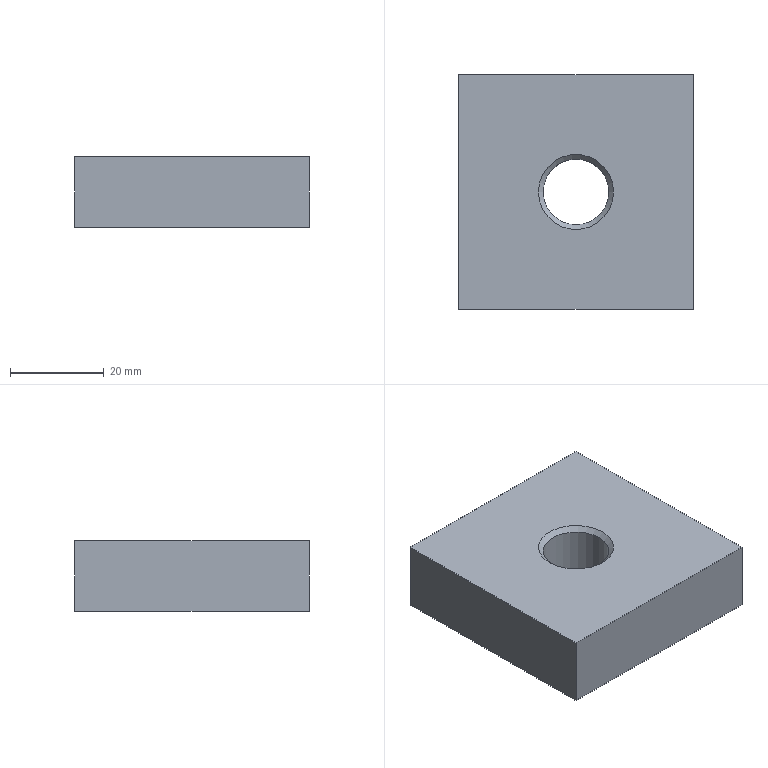Part | STEP file | Spacer block | 1 solid | 9 faces | box 50 x 50 x 15 mm | volume 35145 mm3 | plane 6 | cone 2 | cylinder 1 | commonest cylinder face diameters 14 x1
STEP:
#1=CARTESIAN_POINT('',(0.,0.,0.));
#2=DIRECTION('',(0.,0.,1.));
#3=DIRECTION('',(1.,0.,0.));
#4=AXIS2_PLACEMENT_3D('',#1,#2,#3);
#5=CARTESIAN_POINT('',(-803.5,375.,-765.));
#6=VERTEX_POINT('',#5);
#7=CARTESIAN_POINT('',(-803.5,425.,-765.));
#8=VERTEX_POINT('',#7);
#9=CARTESIAN_POINT('',(-803.5,80.,-765.));
#10=DIRECTION('',(0.,1.,0.));
#11=VECTOR('',#10,1.);
#12=LINE('',#9,#11);
#13=CARTESIAN_POINT('',(-803.5,380.,-640.));
#14=DIRECTION('',(1.,0.,0.));
#15=DIRECTION('',(0.,1.,0.));
#16=AXIS2_PLACEMENT_3D('',#13,#14,#15);
#17=PLANE('',#16);
#18=CARTESIAN_POINT('',(-300.,-125.));
#19=DIRECTION('',(1.,0.));
#20=VECTOR('',#19,1.);
#21=LINE('',#18,#20);
#22=(GEOMETRIC_REPRESENTATION_CONTEXT(2)PARAMETRIC_REPRESENTATION_CONTEXT()REPRESENTATION_CONTEXT('',''));
#23=DEFINITIONAL_REPRESENTATION('',(#21),#22);
#24=PCURVE('',#17,#23);
#25=CARTESIAN_POINT('',(-1203.5,80.,-765.));
#26=DIRECTION('',(0.,0.,-1.));
#27=DIRECTION('',(-1.,0.,0.));
#28=AXIS2_PLACEMENT_3D('',#25,#26,#27);
#29=PLANE('',#28);
#30=CARTESIAN_POINT('',(-400.,0.));
#31=DIRECTION('',(0.,1.));
#32=VECTOR('',#31,1.);
#33=LINE('',#30,#32);
#34=(GEOMETRIC_REPRESENTATION_CONTEXT(2)PARAMETRIC_REPRESENTATION_CONTEXT()REPRESENTATION_CONTEXT('',''));
#35=DEFINITIONAL_REPRESENTATION('',(#33),#34);
#36=PCURVE('',#29,#35);
#37=SURFACE_CURVE('',#12,(#24,#36),.PCURVE_S1.);
#38=EDGE_CURVE('',#6,#8,#37,.T.);
#39=ORIENTED_EDGE('',*,*,#38,.F.);
#40=CARTESIAN_POINT('',(-803.5,375.,-750.));
#41=VERTEX_POINT('',#40);
#42=CARTESIAN_POINT('',(-803.5,375.,-640.));
#43=DIRECTION('',(0.,0.,1.));
#44=VECTOR('',#43,1.);
#45=LINE('',#42,#44);
#46=CARTESIAN_POINT('',(-5.,0.));
#47=DIRECTION('',(0.,1.));
#48=VECTOR('',#47,1.);
#49=LINE('',#46,#48);
#50=(GEOMETRIC_REPRESENTATION_CONTEXT(2)PARAMETRIC_REPRESENTATION_CONTEXT()REPRESENTATION_CONTEXT('',''));
#51=DEFINITIONAL_REPRESENTATION('',(#49),#50);
#52=PCURVE('',#17,#51);
#53=CARTESIAN_POINT('',(-758.5,375.,-640.));
#54=DIRECTION('',(0.,1.,0.));
#55=DIRECTION('',(-1.,0.,0.));
#56=AXIS2_PLACEMENT_3D('',#53,#54,#55);
#57=PLANE('',#56);
#58=CARTESIAN_POINT('',(45.,0.));
#59=DIRECTION('',(0.,1.));
#60=VECTOR('',#59,1.);
#61=LINE('',#58,#60);
#62=(GEOMETRIC_REPRESENTATION_CONTEXT(2)PARAMETRIC_REPRESENTATION_CONTEXT()REPRESENTATION_CONTEXT('',''));
#63=DEFINITIONAL_REPRESENTATION('',(#61),#62);
#64=PCURVE('',#57,#63);
#65=SURFACE_CURVE('',#45,(#52,#64),.PCURVE_S1.);
#66=EDGE_CURVE('',#6,#41,#65,.T.);
#67=ORIENTED_EDGE('',*,*,#66,.T.);
#68=CARTESIAN_POINT('',(-803.5,425.,-750.));
#69=VERTEX_POINT('',#68);
#70=CARTESIAN_POINT('',(-803.5,80.,-750.));
#71=DIRECTION('',(0.,1.,0.));
#72=VECTOR('',#71,1.);
#73=LINE('',#70,#72);
#74=CARTESIAN_POINT('',(-300.,-110.));
#75=DIRECTION('',(1.,0.));
#76=VECTOR('',#75,1.);
#77=LINE('',#74,#76);
#78=(GEOMETRIC_REPRESENTATION_CONTEXT(2)PARAMETRIC_REPRESENTATION_CONTEXT()REPRESENTATION_CONTEXT('',''));
#79=DEFINITIONAL_REPRESENTATION('',(#77),#78);
#80=PCURVE('',#17,#79);
#81=CARTESIAN_POINT('',(-1203.5,80.,-750.));
#82=DIRECTION('',(0.,0.,-1.));
#83=DIRECTION('',(-1.,0.,0.));
#84=AXIS2_PLACEMENT_3D('',#81,#82,#83);
#85=PLANE('',#84);
#86=CARTESIAN_POINT('',(-400.,0.));
#87=DIRECTION('',(0.,1.));
#88=VECTOR('',#87,1.);
#89=LINE('',#86,#88);
#90=(GEOMETRIC_REPRESENTATION_CONTEXT(2)PARAMETRIC_REPRESENTATION_CONTEXT()REPRESENTATION_CONTEXT('',''));
#91=DEFINITIONAL_REPRESENTATION('',(#89),#90);
#92=PCURVE('',#85,#91);
#93=SURFACE_CURVE('',#73,(#80,#92),.PCURVE_S1.);
#94=EDGE_CURVE('',#41,#69,#93,.T.);
#95=ORIENTED_EDGE('',*,*,#94,.T.);
#96=CARTESIAN_POINT('',(-803.5,425.,-640.));
#97=DIRECTION('',(0.,0.,1.));
#98=VECTOR('',#97,1.);
#99=LINE('',#96,#98);
#100=CARTESIAN_POINT('',(45.,0.));
#101=DIRECTION('',(0.,1.));
#102=VECTOR('',#101,1.);
#103=LINE('',#100,#102);
#104=(GEOMETRIC_REPRESENTATION_CONTEXT(2)PARAMETRIC_REPRESENTATION_CONTEXT()REPRESENTATION_CONTEXT('',''));
#105=DEFINITIONAL_REPRESENTATION('',(#103),#104);
#106=PCURVE('',#17,#105);
#107=CARTESIAN_POINT('',(-798.5,425.,-640.));
#108=DIRECTION('',(0.,-1.,0.));
#109=DIRECTION('',(0.,0.,-1.));
#110=AXIS2_PLACEMENT_3D('',#107,#108,#109);
#111=PLANE('',#110);
#112=CARTESIAN_POINT('',(0.,-5.));
#113=DIRECTION('',(-1.,0.));
#114=VECTOR('',#113,1.);
#115=LINE('',#112,#114);
#116=(GEOMETRIC_REPRESENTATION_CONTEXT(2)PARAMETRIC_REPRESENTATION_CONTEXT()REPRESENTATION_CONTEXT('',''));
#117=DEFINITIONAL_REPRESENTATION('',(#115),#116);
#118=PCURVE('',#111,#117);
#119=SURFACE_CURVE('',#99,(#106,#118),.PCURVE_S1.);
#120=EDGE_CURVE('',#8,#69,#119,.T.);
#121=ORIENTED_EDGE('',*,*,#120,.F.);
#122=EDGE_LOOP('',(#39,#67,#95,#121));
#123=FACE_BOUND('',#122,.T.);
#124=ADVANCED_FACE('',(#123),#17,.F.);
#125=CARTESIAN_POINT('',(-753.5,375.,-765.));
#126=VERTEX_POINT('',#125);
#127=CARTESIAN_POINT('',(-1203.5,375.,-765.));
#128=DIRECTION('',(-1.,0.,0.));
#129=VECTOR('',#128,1.);
#130=LINE('',#127,#129);
#131=CARTESIAN_POINT('',(445.,-125.));
#132=DIRECTION('',(1.,0.));
#133=VECTOR('',#132,1.);
#134=LINE('',#131,#133);
#135=(GEOMETRIC_REPRESENTATION_CONTEXT(2)PARAMETRIC_REPRESENTATION_CONTEXT()REPRESENTATION_CONTEXT('',''));
#136=DEFINITIONAL_REPRESENTATION('',(#134),#135);
#137=PCURVE('',#57,#136);
#138=CARTESIAN_POINT('',(0.,295.));
#139=DIRECTION('',(1.,0.));
#140=VECTOR('',#139,1.);
#141=LINE('',#138,#140);
#142=(GEOMETRIC_REPRESENTATION_CONTEXT(2)PARAMETRIC_REPRESENTATION_CONTEXT()REPRESENTATION_CONTEXT('',''));
#143=DEFINITIONAL_REPRESENTATION('',(#141),#142);
#144=PCURVE('',#29,#143);
#145=SURFACE_CURVE('',#130,(#137,#144),.PCURVE_S1.);
#146=EDGE_CURVE('',#126,#6,#145,.T.);
#147=ORIENTED_EDGE('',*,*,#146,.F.);
#148=CARTESIAN_POINT('',(-753.5,375.,-750.));
#149=VERTEX_POINT('',#148);
#150=CARTESIAN_POINT('',(-753.5,375.,-640.));
#151=DIRECTION('',(0.,0.,1.));
#152=VECTOR('',#151,1.);
#153=LINE('',#150,#152);
#154=CARTESIAN_POINT('',(-5.,0.));
#155=DIRECTION('',(0.,1.));
#156=VECTOR('',#155,1.);
#157=LINE('',#154,#156);
#158=(GEOMETRIC_REPRESENTATION_CONTEXT(2)PARAMETRIC_REPRESENTATION_CONTEXT()REPRESENTATION_CONTEXT('',''));
#159=DEFINITIONAL_REPRESENTATION('',(#157),#158);
#160=PCURVE('',#57,#159);
#161=CARTESIAN_POINT('',(-753.5,420.,-640.));
#162=DIRECTION('',(-1.,0.,0.));
#163=DIRECTION('',(0.,0.,1.));
#164=AXIS2_PLACEMENT_3D('',#161,#162,#163);
#165=PLANE('',#164);
#166=CARTESIAN_POINT('',(0.,-45.));
#167=DIRECTION('',(1.,0.));
#168=VECTOR('',#167,1.);
#169=LINE('',#166,#168);
#170=(GEOMETRIC_REPRESENTATION_CONTEXT(2)PARAMETRIC_REPRESENTATION_CONTEXT()REPRESENTATION_CONTEXT('',''));
#171=DEFINITIONAL_REPRESENTATION('',(#169),#170);
#172=PCURVE('',#165,#171);
#173=SURFACE_CURVE('',#153,(#160,#172),.PCURVE_S1.);
#174=EDGE_CURVE('',#126,#149,#173,.T.);
#175=ORIENTED_EDGE('',*,*,#174,.T.);
#176=CARTESIAN_POINT('',(-1203.5,375.,-750.));
#177=DIRECTION('',(-1.,0.,0.));
#178=VECTOR('',#177,1.);
#179=LINE('',#176,#178);
#180=CARTESIAN_POINT('',(445.,-110.));
#181=DIRECTION('',(1.,0.));
#182=VECTOR('',#181,1.);
#183=LINE('',#180,#182);
#184=(GEOMETRIC_REPRESENTATION_CONTEXT(2)PARAMETRIC_REPRESENTATION_CONTEXT()REPRESENTATION_CONTEXT('',''));
#185=DEFINITIONAL_REPRESENTATION('',(#183),#184);
#186=PCURVE('',#57,#185);
#187=CARTESIAN_POINT('',(0.,295.));
#188=DIRECTION('',(1.,0.));
#189=VECTOR('',#188,1.);
#190=LINE('',#187,#189);
#191=(GEOMETRIC_REPRESENTATION_CONTEXT(2)PARAMETRIC_REPRESENTATION_CONTEXT()REPRESENTATION_CONTEXT('',''));
#192=DEFINITIONAL_REPRESENTATION('',(#190),#191);
#193=PCURVE('',#85,#192);
#194=SURFACE_CURVE('',#179,(#186,#193),.PCURVE_S1.);
#195=EDGE_CURVE('',#149,#41,#194,.T.);
#196=ORIENTED_EDGE('',*,*,#195,.T.);
#197=ORIENTED_EDGE('',*,*,#66,.F.);
#198=EDGE_LOOP('',(#147,#175,#196,#197));
#199=FACE_BOUND('',#198,.T.);
#200=ADVANCED_FACE('',(#199),#57,.F.);
#201=CARTESIAN_POINT('',(-753.5,425.,-765.));
#202=VERTEX_POINT('',#201);
#203=CARTESIAN_POINT('',(-753.5,80.,-765.));
#204=DIRECTION('',(0.,-1.,0.));
#205=VECTOR('',#204,1.);
#206=LINE('',#203,#205);
#207=CARTESIAN_POINT('',(-125.,-340.));
#208=DIRECTION('',(0.,-1.));
#209=VECTOR('',#208,1.);
#210=LINE('',#207,#209);
#211=(GEOMETRIC_REPRESENTATION_CONTEXT(2)PARAMETRIC_REPRESENTATION_CONTEXT()REPRESENTATION_CONTEXT('',''));
#212=DEFINITIONAL_REPRESENTATION('',(#210),#211);
#213=PCURVE('',#165,#212);
#214=CARTESIAN_POINT('',(-450.,0.));
#215=DIRECTION('',(0.,-1.));
#216=VECTOR('',#215,1.);
#217=LINE('',#214,#216);
#218=(GEOMETRIC_REPRESENTATION_CONTEXT(2)PARAMETRIC_REPRESENTATION_CONTEXT()REPRESENTATION_CONTEXT('',''));
#219=DEFINITIONAL_REPRESENTATION('',(#217),#218);
#220=PCURVE('',#29,#219);
#221=SURFACE_CURVE('',#206,(#213,#220),.PCURVE_S1.);
#222=EDGE_CURVE('',#202,#126,#221,.T.);
#223=ORIENTED_EDGE('',*,*,#222,.F.);
#224=CARTESIAN_POINT('',(-753.5,425.,-750.));
#225=VERTEX_POINT('',#224);
#226=CARTESIAN_POINT('',(-753.5,425.,-640.));
#227=DIRECTION('',(0.,0.,1.));
#228=VECTOR('',#227,1.);
#229=LINE('',#226,#228);
#230=CARTESIAN_POINT('',(0.,5.));
#231=DIRECTION('',(1.,0.));
#232=VECTOR('',#231,1.);
#233=LINE('',#230,#232);
#234=(GEOMETRIC_REPRESENTATION_CONTEXT(2)PARAMETRIC_REPRESENTATION_CONTEXT()REPRESENTATION_CONTEXT('',''));
#235=DEFINITIONAL_REPRESENTATION('',(#233),#234);
#236=PCURVE('',#165,#235);
#237=CARTESIAN_POINT('',(0.,45.));
#238=DIRECTION('',(-1.,0.));
#239=VECTOR('',#238,1.);
#240=LINE('',#237,#239);
#241=(GEOMETRIC_REPRESENTATION_CONTEXT(2)PARAMETRIC_REPRESENTATION_CONTEXT()REPRESENTATION_CONTEXT('',''));
#242=DEFINITIONAL_REPRESENTATION('',(#240),#241);
#243=PCURVE('',#111,#242);
#244=SURFACE_CURVE('',#229,(#236,#243),.PCURVE_S1.);
#245=EDGE_CURVE('',#202,#225,#244,.T.);
#246=ORIENTED_EDGE('',*,*,#245,.T.);
#247=CARTESIAN_POINT('',(-753.5,80.,-750.));
#248=DIRECTION('',(0.,-1.,0.));
#249=VECTOR('',#248,1.);
#250=LINE('',#247,#249);
#251=CARTESIAN_POINT('',(-110.,-340.));
#252=DIRECTION('',(0.,-1.));
#253=VECTOR('',#252,1.);
#254=LINE('',#251,#253);
#255=(GEOMETRIC_REPRESENTATION_CONTEXT(2)PARAMETRIC_REPRESENTATION_CONTEXT()REPRESENTATION_CONTEXT('',''));
#256=DEFINITIONAL_REPRESENTATION('',(#254),#255);
#257=PCURVE('',#165,#256);
#258=CARTESIAN_POINT('',(-450.,0.));
#259=DIRECTION('',(0.,-1.));
#260=VECTOR('',#259,1.);
#261=LINE('',#258,#260);
#262=(GEOMETRIC_REPRESENTATION_CONTEXT(2)PARAMETRIC_REPRESENTATION_CONTEXT()REPRESENTATION_CONTEXT('',''));
#263=DEFINITIONAL_REPRESENTATION('',(#261),#262);
#264=PCURVE('',#85,#263);
#265=SURFACE_CURVE('',#250,(#257,#264),.PCURVE_S1.);
#266=EDGE_CURVE('',#225,#149,#265,.T.);
#267=ORIENTED_EDGE('',*,*,#266,.T.);
#268=ORIENTED_EDGE('',*,*,#174,.F.);
#269=EDGE_LOOP('',(#223,#246,#267,#268));
#270=FACE_BOUND('',#269,.T.);
#271=ADVANCED_FACE('',(#270),#165,.F.);
#272=CARTESIAN_POINT('',(-1203.5,425.,-765.));
#273=DIRECTION('',(1.,0.,0.));
#274=VECTOR('',#273,1.);
#275=LINE('',#272,#274);
#276=CARTESIAN_POINT('',(125.,-405.));
#277=DIRECTION('',(0.,1.));
#278=VECTOR('',#277,1.);
#279=LINE('',#276,#278);
#280=(GEOMETRIC_REPRESENTATION_CONTEXT(2)PARAMETRIC_REPRESENTATION_CONTEXT()REPRESENTATION_CONTEXT('',''));
#281=DEFINITIONAL_REPRESENTATION('',(#279),#280);
#282=PCURVE('',#111,#281);
#283=CARTESIAN_POINT('',(0.,345.));
#284=DIRECTION('',(-1.,0.));
#285=VECTOR('',#284,1.);
#286=LINE('',#283,#285);
#287=(GEOMETRIC_REPRESENTATION_CONTEXT(2)PARAMETRIC_REPRESENTATION_CONTEXT()REPRESENTATION_CONTEXT('',''));
#288=DEFINITIONAL_REPRESENTATION('',(#286),#287);
#289=PCURVE('',#29,#288);
#290=SURFACE_CURVE('',#275,(#282,#289),.PCURVE_S1.);
#291=EDGE_CURVE('',#8,#202,#290,.T.);
#292=ORIENTED_EDGE('',*,*,#291,.F.);
#293=ORIENTED_EDGE('',*,*,#120,.T.);
#294=CARTESIAN_POINT('',(-1203.5,425.,-750.));
#295=DIRECTION('',(1.,0.,0.));
#296=VECTOR('',#295,1.);
#297=LINE('',#294,#296);
#298=CARTESIAN_POINT('',(110.,-405.));
#299=DIRECTION('',(0.,1.));
#300=VECTOR('',#299,1.);
#301=LINE('',#298,#300);
#302=(GEOMETRIC_REPRESENTATION_CONTEXT(2)PARAMETRIC_REPRESENTATION_CONTEXT()REPRESENTATION_CONTEXT('',''));
#303=DEFINITIONAL_REPRESENTATION('',(#301),#302);
#304=PCURVE('',#111,#303);
#305=CARTESIAN_POINT('',(0.,345.));
#306=DIRECTION('',(-1.,0.));
#307=VECTOR('',#306,1.);
#308=LINE('',#305,#307);
#309=(GEOMETRIC_REPRESENTATION_CONTEXT(2)PARAMETRIC_REPRESENTATION_CONTEXT()REPRESENTATION_CONTEXT('',''));
#310=DEFINITIONAL_REPRESENTATION('',(#308),#309);
#311=PCURVE('',#85,#310);
#312=SURFACE_CURVE('',#297,(#304,#311),.PCURVE_S1.);
#313=EDGE_CURVE('',#69,#225,#312,.T.);
#314=ORIENTED_EDGE('',*,*,#313,.T.);
#315=ORIENTED_EDGE('',*,*,#245,.F.);
#316=EDGE_LOOP('',(#292,#293,#314,#315));
#317=FACE_BOUND('',#316,.T.);
#318=ADVANCED_FACE('',(#317),#111,.F.);
#319=CARTESIAN_POINT('',(-786.5,400.,-750.));
#320=VERTEX_POINT('',#319);
#321=CARTESIAN_POINT('',(-778.5,400.,-750.));
#322=DIRECTION('',(0.,0.,-1.));
#323=DIRECTION('',(-1.,0.,0.));
#324=AXIS2_PLACEMENT_3D('',#321,#322,#323);
#325=CIRCLE('',#324,8.);
#326=CARTESIAN_POINT('',(-425.,320.));
#327=DIRECTION('',(1.,0.));
#328=AXIS2_PLACEMENT_2D('',#326,#327);
#329=CIRCLE('',#328,8.);
#330=(GEOMETRIC_REPRESENTATION_CONTEXT(2)PARAMETRIC_REPRESENTATION_CONTEXT()REPRESENTATION_CONTEXT('',''));
#331=DEFINITIONAL_REPRESENTATION('',(#329),#330);
#332=PCURVE('',#85,#331);
#333=CARTESIAN_POINT('',(-778.5,400.,-750.));
#334=DIRECTION('',(0.,0.,1.));
#335=DIRECTION('',(1.,0.,0.));
#336=AXIS2_PLACEMENT_3D('',#333,#334,#335);
#337=CONICAL_SURFACE('',#336,8.,0.7854);
#338=CARTESIAN_POINT('',(9.425,0.));
#339=DIRECTION('',(-1.,0.));
#340=VECTOR('',#339,1.);
#341=LINE('',#338,#340);
#342=(GEOMETRIC_REPRESENTATION_CONTEXT(2)PARAMETRIC_REPRESENTATION_CONTEXT()REPRESENTATION_CONTEXT('',''));
#343=DEFINITIONAL_REPRESENTATION('',(#341),#342);
#344=PCURVE('',#337,#343);
#345=SURFACE_CURVE('',#325,(#332,#344),.PCURVE_S1.);
#346=EDGE_CURVE('',#320,#320,#345,.T.);
#347=ORIENTED_EDGE('',*,*,#346,.T.);
#348=EDGE_LOOP('',(#347));
#349=FACE_BOUND('',#348,.T.);
#350=ORIENTED_EDGE('',*,*,#94,.F.);
#351=ORIENTED_EDGE('',*,*,#195,.F.);
#352=ORIENTED_EDGE('',*,*,#266,.F.);
#353=ORIENTED_EDGE('',*,*,#313,.F.);
#354=EDGE_LOOP('',(#350,#351,#352,#353));
#355=FACE_BOUND('',#354,.T.);
#356=ADVANCED_FACE('',(#349,#355),#85,.F.);
#357=CARTESIAN_POINT('',(-786.5,400.,-765.));
#358=VERTEX_POINT('',#357);
#359=CARTESIAN_POINT('',(-778.5,400.,-765.));
#360=DIRECTION('',(0.,0.,1.));
#361=DIRECTION('',(-1.,0.,0.));
#362=AXIS2_PLACEMENT_3D('',#359,#360,#361);
#363=CIRCLE('',#362,8.);
#364=CARTESIAN_POINT('',(-417.,320.));
#365=CARTESIAN_POINT('',(-417.,306.144));
#366=CARTESIAN_POINT('',(-429.,313.072));
#367=CARTESIAN_POINT('',(-441.,320.));
#368=CARTESIAN_POINT('',(-429.,326.928));
#369=CARTESIAN_POINT('',(-417.,333.856));
#370=CARTESIAN_POINT('',(-417.,320.));
#371=(BOUNDED_CURVE()B_SPLINE_CURVE(2,(#364,#365,#366,#367,#368,#369,#370),.UNSPECIFIED.,.T.,.F.)B_SPLINE_CURVE_WITH_KNOTS((1,2,2,2,2,1),(-2.094,0.,2.094,4.189,6.283,8.378),.UNSPECIFIED.)CURVE()GEOMETRIC_REPRESENTATION_ITEM()RATIONAL_B_SPLINE_CURVE((1.,0.5,1.,0.5,1.,0.5,1.))REPRESENTATION_ITEM(''));
#372=(GEOMETRIC_REPRESENTATION_CONTEXT(2)PARAMETRIC_REPRESENTATION_CONTEXT()REPRESENTATION_CONTEXT('',''));
#373=DEFINITIONAL_REPRESENTATION('',(#371),#372);
#374=PCURVE('',#29,#373);
#375=CARTESIAN_POINT('',(-778.5,400.,-765.));
#376=DIRECTION('',(0.,0.,-1.));
#377=DIRECTION('',(-1.,0.,0.));
#378=AXIS2_PLACEMENT_3D('',#375,#376,#377);
#379=CONICAL_SURFACE('',#378,8.,0.7854);
#380=CARTESIAN_POINT('',(6.283,0.));
#381=DIRECTION('',(-1.,0.));
#382=VECTOR('',#381,1.);
#383=LINE('',#380,#382);
#384=(GEOMETRIC_REPRESENTATION_CONTEXT(2)PARAMETRIC_REPRESENTATION_CONTEXT()REPRESENTATION_CONTEXT('',''));
#385=DEFINITIONAL_REPRESENTATION('',(#383),#384);
#386=PCURVE('',#379,#385);
#387=SURFACE_CURVE('',#363,(#374,#386),.PCURVE_S1.);
#388=EDGE_CURVE('',#358,#358,#387,.T.);
#389=ORIENTED_EDGE('',*,*,#388,.T.);
#390=EDGE_LOOP('',(#389));
#391=FACE_BOUND('',#390,.T.);
#392=ORIENTED_EDGE('',*,*,#38,.T.);
#393=ORIENTED_EDGE('',*,*,#291,.T.);
#394=ORIENTED_EDGE('',*,*,#222,.T.);
#395=ORIENTED_EDGE('',*,*,#146,.T.);
#396=EDGE_LOOP('',(#392,#393,#394,#395));
#397=FACE_BOUND('',#396,.T.);
#398=ADVANCED_FACE('',(#391,#397),#29,.T.);
#399=CARTESIAN_POINT('',(-785.5,400.,-751.));
#400=VERTEX_POINT('',#399);
#401=CARTESIAN_POINT('',(-778.5,400.,-751.));
#402=DIRECTION('',(0.,0.,1.));
#403=DIRECTION('',(-1.,0.,0.));
#404=AXIS2_PLACEMENT_3D('',#401,#402,#403);
#405=CIRCLE('',#404,7.);
#406=CARTESIAN_POINT('',(-778.5,400.,-765.));
#407=DIRECTION('',(0.,0.,1.));
#408=DIRECTION('',(1.,0.,0.));
#409=AXIS2_PLACEMENT_3D('',#406,#407,#408);
#410=CYLINDRICAL_SURFACE('',#409,7.);
#411=CARTESIAN_POINT('',(3.142,14.));
#412=DIRECTION('',(1.,0.));
#413=VECTOR('',#412,1.);
#414=LINE('',#411,#413);
#415=(GEOMETRIC_REPRESENTATION_CONTEXT(2)PARAMETRIC_REPRESENTATION_CONTEXT()REPRESENTATION_CONTEXT('',''));
#416=DEFINITIONAL_REPRESENTATION('',(#414),#415);
#417=PCURVE('',#410,#416);
#418=CARTESIAN_POINT('',(3.142,-1.));
#419=DIRECTION('',(1.,0.));
#420=VECTOR('',#419,1.);
#421=LINE('',#418,#420);
#422=(GEOMETRIC_REPRESENTATION_CONTEXT(2)PARAMETRIC_REPRESENTATION_CONTEXT()REPRESENTATION_CONTEXT('',''));
#423=DEFINITIONAL_REPRESENTATION('',(#421),#422);
#424=PCURVE('',#337,#423);
#425=SURFACE_CURVE('',#405,(#417,#424),.PCURVE_S1.);
#426=EDGE_CURVE('',#400,#400,#425,.T.);
#427=ORIENTED_EDGE('',*,*,#426,.F.);
#428=CARTESIAN_POINT('',(-785.5,400.,-764.));
#429=VERTEX_POINT('',#428);
#430=CARTESIAN_POINT('',(-785.5,400.,-764.));
#431=CARTESIAN_POINT('',(-785.5,400.,-751.));
#432=B_SPLINE_CURVE_WITH_KNOTS('',1,(#430,#431),.UNSPECIFIED.,.F.,.F.,(2,2),(1.,14.),.PIECEWISE_BEZIER_KNOTS.);
#433=CARTESIAN_POINT('',(3.142,0.));
#434=DIRECTION('',(0.,1.));
#435=VECTOR('',#434,1.);
#436=LINE('',#433,#435);
#437=(GEOMETRIC_REPRESENTATION_CONTEXT(2)PARAMETRIC_REPRESENTATION_CONTEXT()REPRESENTATION_CONTEXT('',''));
#438=DEFINITIONAL_REPRESENTATION('',(#436),#437);
#439=PCURVE('',#410,#438);
#440=CARTESIAN_POINT('',(9.425,0.));
#441=DIRECTION('',(0.,1.));
#442=VECTOR('',#441,1.);
#443=LINE('',#440,#442);
#444=(GEOMETRIC_REPRESENTATION_CONTEXT(2)PARAMETRIC_REPRESENTATION_CONTEXT()REPRESENTATION_CONTEXT('',''));
#445=DEFINITIONAL_REPRESENTATION('',(#443),#444);
#446=PCURVE('',#410,#445);
#447=SEAM_CURVE('',#432,(#439,#446),.PCURVE_S1.);
#448=EDGE_CURVE('',#429,#400,#447,.T.);
#449=ORIENTED_EDGE('',*,*,#448,.F.);
#450=CARTESIAN_POINT('',(-778.5,400.,-764.));
#451=DIRECTION('',(0.,0.,-1.));
#452=DIRECTION('',(-1.,0.,0.));
#453=AXIS2_PLACEMENT_3D('',#450,#451,#452);
#454=CIRCLE('',#453,7.);
#455=CARTESIAN_POINT('',(9.425,1.));
#456=DIRECTION('',(-1.,0.));
#457=VECTOR('',#456,1.);
#458=LINE('',#455,#457);
#459=(GEOMETRIC_REPRESENTATION_CONTEXT(2)PARAMETRIC_REPRESENTATION_CONTEXT()REPRESENTATION_CONTEXT('',''));
#460=DEFINITIONAL_REPRESENTATION('',(#458),#459);
#461=PCURVE('',#410,#460);
#462=CARTESIAN_POINT('',(0.,-1.));
#463=DIRECTION('',(1.,0.));
#464=VECTOR('',#463,1.);
#465=LINE('',#462,#464);
#466=(GEOMETRIC_REPRESENTATION_CONTEXT(2)PARAMETRIC_REPRESENTATION_CONTEXT()REPRESENTATION_CONTEXT('',''));
#467=DEFINITIONAL_REPRESENTATION('',(#465),#466);
#468=PCURVE('',#379,#467);
#469=SURFACE_CURVE('',#454,(#461,#468),.PCURVE_S1.);
#470=EDGE_CURVE('',#429,#429,#469,.T.);
#471=ORIENTED_EDGE('',*,*,#470,.F.);
#472=ORIENTED_EDGE('',*,*,#448,.T.);
#473=EDGE_LOOP('',(#427,#449,#471,#472));
#474=FACE_BOUND('',#473,.F.);
#475=ADVANCED_FACE('',(#474),#410,.F.);
#476=ORIENTED_EDGE('',*,*,#470,.T.);
#477=CARTESIAN_POINT('',(-785.5,400.,-764.));
#478=CARTESIAN_POINT('',(-786.5,400.,-765.));
#479=B_SPLINE_CURVE_WITH_KNOTS('',1,(#477,#478),.UNSPECIFIED.,.F.,.F.,(2,2),(-1.414,0.),.PIECEWISE_BEZIER_KNOTS.);
#480=CARTESIAN_POINT('',(6.283,0.));
#481=DIRECTION('',(0.,1.));
#482=VECTOR('',#481,1.);
#483=LINE('',#480,#482);
#484=(GEOMETRIC_REPRESENTATION_CONTEXT(2)PARAMETRIC_REPRESENTATION_CONTEXT()REPRESENTATION_CONTEXT('',''));
#485=DEFINITIONAL_REPRESENTATION('',(#483),#484);
#486=PCURVE('',#379,#485);
#487=CARTESIAN_POINT('',(0.,0.));
#488=DIRECTION('',(0.,1.));
#489=VECTOR('',#488,1.);
#490=LINE('',#487,#489);
#491=(GEOMETRIC_REPRESENTATION_CONTEXT(2)PARAMETRIC_REPRESENTATION_CONTEXT()REPRESENTATION_CONTEXT('',''));
#492=DEFINITIONAL_REPRESENTATION('',(#490),#491);
#493=PCURVE('',#379,#492);
#494=SEAM_CURVE('',#479,(#486,#493),.PCURVE_S1.);
#495=EDGE_CURVE('',#429,#358,#494,.T.);
#496=ORIENTED_EDGE('',*,*,#495,.T.);
#497=ORIENTED_EDGE('',*,*,#388,.T.);
#498=ORIENTED_EDGE('',*,*,#495,.F.);
#499=EDGE_LOOP('',(#476,#496,#497,#498));
#500=FACE_BOUND('',#499,.F.);
#501=ADVANCED_FACE('',(#500),#379,.F.);
#502=ORIENTED_EDGE('',*,*,#426,.T.);
#503=CARTESIAN_POINT('',(-785.5,400.,-751.));
#504=CARTESIAN_POINT('',(-786.5,400.,-750.));
#505=B_SPLINE_CURVE_WITH_KNOTS('',1,(#503,#504),.UNSPECIFIED.,.F.,.F.,(2,2),(-1.414,0.),.PIECEWISE_BEZIER_KNOTS.);
#506=CARTESIAN_POINT('',(9.425,0.));
#507=DIRECTION('',(0.,1.));
#508=VECTOR('',#507,1.);
#509=LINE('',#506,#508);
#510=(GEOMETRIC_REPRESENTATION_CONTEXT(2)PARAMETRIC_REPRESENTATION_CONTEXT()REPRESENTATION_CONTEXT('',''));
#511=DEFINITIONAL_REPRESENTATION('',(#509),#510);
#512=PCURVE('',#337,#511);
#513=CARTESIAN_POINT('',(3.142,0.));
#514=DIRECTION('',(0.,1.));
#515=VECTOR('',#514,1.);
#516=LINE('',#513,#515);
#517=(GEOMETRIC_REPRESENTATION_CONTEXT(2)PARAMETRIC_REPRESENTATION_CONTEXT()REPRESENTATION_CONTEXT('',''));
#518=DEFINITIONAL_REPRESENTATION('',(#516),#517);
#519=PCURVE('',#337,#518);
#520=SEAM_CURVE('',#505,(#512,#519),.PCURVE_S1.);
#521=EDGE_CURVE('',#400,#320,#520,.T.);
#522=ORIENTED_EDGE('',*,*,#521,.T.);
#523=ORIENTED_EDGE('',*,*,#346,.T.);
#524=ORIENTED_EDGE('',*,*,#521,.F.);
#525=EDGE_LOOP('',(#502,#522,#523,#524));
#526=FACE_BOUND('',#525,.F.);
#527=ADVANCED_FACE('',(#526),#337,.F.);
#528=CLOSED_SHELL('',(#124,#200,#271,#318,#356,#398,#475,#501,#527));
#529=MANIFOLD_SOLID_BREP('',#528);
#530=(LENGTH_UNIT()NAMED_UNIT(*)SI_UNIT(.MILLI.,.METRE.));
#531=UNCERTAINTY_MEASURE_WITH_UNIT(LENGTH_MEASURE(0.000002),#530,'','');
#532=(NAMED_UNIT(*)PLANE_ANGLE_UNIT()SI_UNIT($,.RADIAN.));
#533=(NAMED_UNIT(*)SI_UNIT($,.STERADIAN.)SOLID_ANGLE_UNIT());
#534=(GEOMETRIC_REPRESENTATION_CONTEXT(3)GLOBAL_UNCERTAINTY_ASSIGNED_CONTEXT((#531))GLOBAL_UNIT_ASSIGNED_CONTEXT((#530,#532,#533))REPRESENTATION_CONTEXT('',''));
#535=ADVANCED_BREP_SHAPE_REPRESENTATION('',(#4,#529),#534);